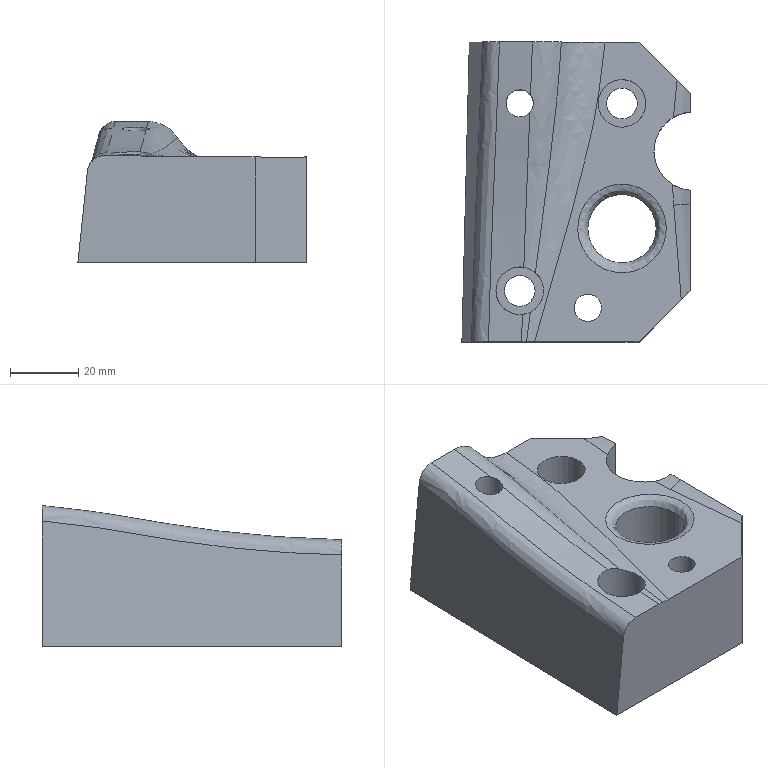Part | NX | features solid 2 | 1 solid | 29 faces | box 66.988 x 88.001 x 41.352 mm | volume 148897 mm3 | spline 11 | plane 9 | cylinder 9 | commonest cylinder face diameters 8 x2 9 x2 14 x2 20.05 x2 23 x1